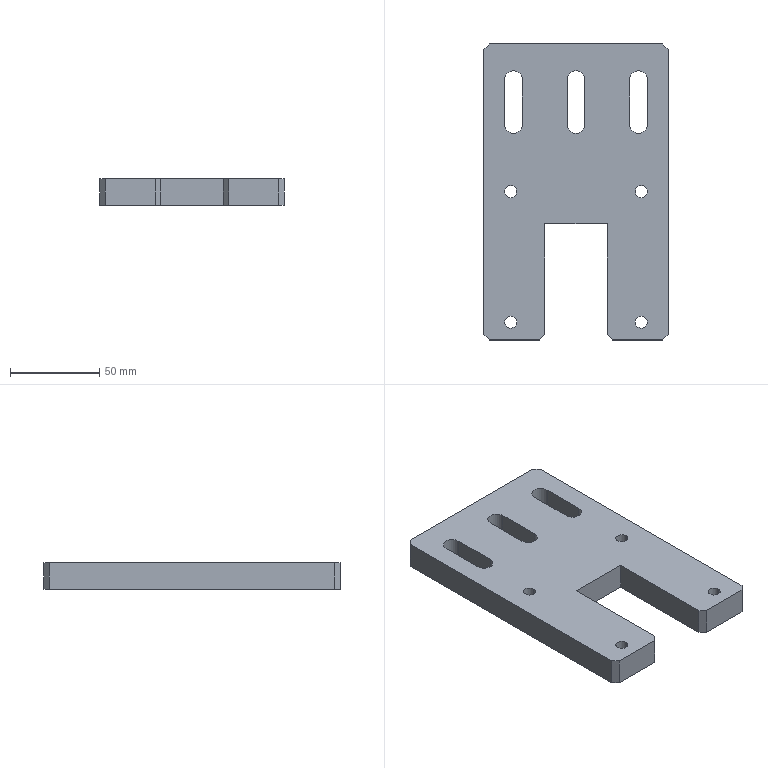Part | STEP file | 1 solid | 36 faces | box 103 x 165.5 x 15 mm | volume 204204 mm3 | plane 22 | cylinder 14 | commonest cylinder face diameters 6.8 x8 10 x6